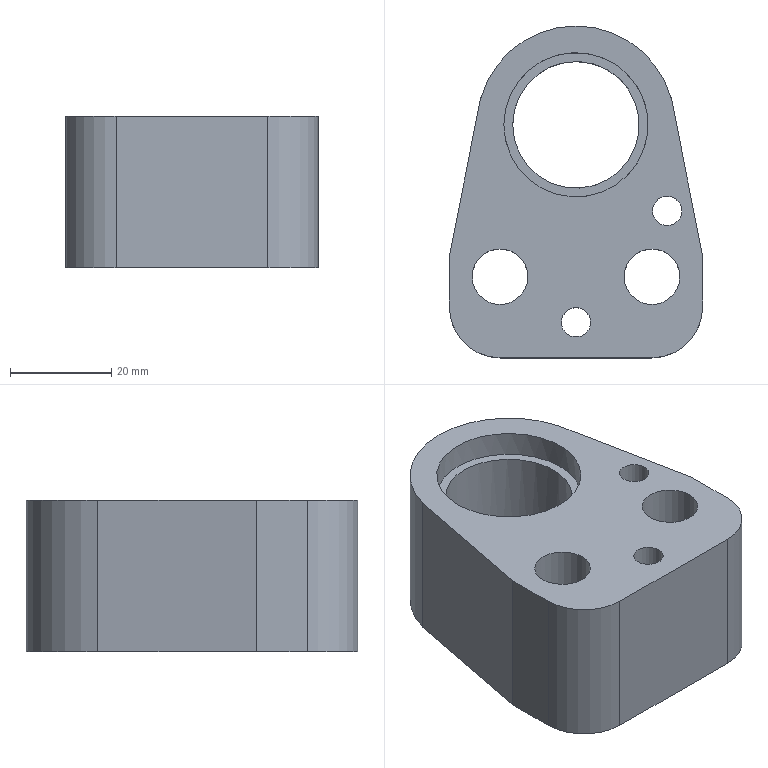Part | NX | features solid 2 | 1 solid | 27 faces | box 50 x 65.5 x 30 mm | volume 54795 mm3 | plane 14 | cylinder 13 | commonest cylinder face diameters 5.8 x2 8 x2 11 x2 17 x2 20 x2 25 x1
STEP:
#1=CARTESIAN_POINT('',(133.569,-304.452,65.));
#2=VERTEX_POINT('',#1);
#3=CARTESIAN_POINT('',(133.569,-304.452,95.));
#4=VERTEX_POINT('',#3);
#5=CARTESIAN_POINT('',(133.569,-304.452,65.));
#6=DIRECTION('',(0.,0.,1.));
#7=VECTOR('',#6,1000.);
#8=LINE('',#5,#7);
#9=EDGE_CURVE('',#2,#4,#8,.T.);
#10=ORIENTED_EDGE('',*,*,#9,.F.);
#11=CARTESIAN_POINT('',(133.497,-304.452,65.));
#12=VERTEX_POINT('',#11);
#13=CARTESIAN_POINT('',(114.754,-304.452,65.));
#14=DIRECTION('',(-1.,0.,0.));
#15=VECTOR('',#14,1000.);
#16=LINE('',#13,#15);
#17=EDGE_CURVE('',#2,#12,#16,.T.);
#18=ORIENTED_EDGE('',*,*,#17,.T.);
#19=CARTESIAN_POINT('',(133.497,-304.452,95.));
#20=VERTEX_POINT('',#19);
#21=CARTESIAN_POINT('',(133.497,-304.452,95.));
#22=DIRECTION('',(0.,0.,-1.));
#23=VECTOR('',#22,1000.);
#24=LINE('',#21,#23);
#25=EDGE_CURVE('',#20,#12,#24,.T.);
#26=ORIENTED_EDGE('',*,*,#25,.F.);
#27=CARTESIAN_POINT('',(114.754,-304.452,95.));
#28=DIRECTION('',(1.,0.,0.));
#29=VECTOR('',#28,1000.);
#30=LINE('',#27,#29);
#31=EDGE_CURVE('',#20,#4,#30,.T.);
#32=ORIENTED_EDGE('',*,*,#31,.T.);
#33=EDGE_LOOP('',(#10,#18,#26,#32));
#34=FACE_BOUND('',#33,.T.);
#35=CARTESIAN_POINT('',(114.754,-304.452,65.));
#36=DIRECTION('',(0.,1.,0.));
#37=DIRECTION('',(0.,0.,1.));
#38=AXIS2_PLACEMENT_3D('',#35,#36,#37);
#39=PLANE('',#38);
#40=ADVANCED_FACE('',(#34),#39,.T.);
#41=CARTESIAN_POINT('',(139.754,-335.832,95.));
#42=VERTEX_POINT('',#41);
#43=CARTESIAN_POINT('',(135.886,-316.209,95.));
#44=DIRECTION('',(-0.1934,0.9811,0.));
#45=VECTOR('',#44,1000.);
#46=LINE('',#43,#45);
#47=EDGE_CURVE('',#42,#4,#46,.T.);
#48=ORIENTED_EDGE('',*,*,#47,.T.);
#49=ORIENTED_EDGE('',*,*,#31,.F.);
#50=CARTESIAN_POINT('',(96.011,-304.452,95.));
#51=VERTEX_POINT('',#50);
#52=CARTESIAN_POINT('',(114.754,-309.832,95.));
#53=DIRECTION('',(0.,0.,-1.));
#54=DIRECTION('',(-1.,0.,0.));
#55=AXIS2_PLACEMENT_3D('',#52,#53,#54);
#56=CIRCLE('',#55,19.5);
#57=EDGE_CURVE('',#51,#20,#56,.T.);
#58=ORIENTED_EDGE('',*,*,#57,.F.);
#59=CARTESIAN_POINT('',(95.939,-304.452,95.));
#60=VERTEX_POINT('',#59);
#61=CARTESIAN_POINT('',(114.754,-304.452,95.));
#62=DIRECTION('',(1.,0.,0.));
#63=VECTOR('',#62,1000.);
#64=LINE('',#61,#63);
#65=EDGE_CURVE('',#60,#51,#64,.T.);
#66=ORIENTED_EDGE('',*,*,#65,.F.);
#67=CARTESIAN_POINT('',(89.754,-335.832,95.));
#68=VERTEX_POINT('',#67);
#69=CARTESIAN_POINT('',(93.622,-316.209,95.));
#70=DIRECTION('',(-0.1934,-0.9811,0.));
#71=VECTOR('',#70,1000.);
#72=LINE('',#69,#71);
#73=EDGE_CURVE('',#60,#68,#72,.T.);
#74=ORIENTED_EDGE('',*,*,#73,.T.);
#75=CARTESIAN_POINT('',(89.754,-345.832,95.));
#76=VERTEX_POINT('',#75);
#77=CARTESIAN_POINT('',(89.754,-320.142,95.));
#78=DIRECTION('',(0.,1.,0.));
#79=VECTOR('',#78,1000.);
#80=LINE('',#77,#79);
#81=EDGE_CURVE('',#76,#68,#80,.T.);
#82=ORIENTED_EDGE('',*,*,#81,.F.);
#83=CARTESIAN_POINT('',(99.754,-355.832,95.));
#84=VERTEX_POINT('',#83);
#85=CARTESIAN_POINT('',(99.754,-345.832,95.));
#86=DIRECTION('',(0.,0.,1.));
#87=DIRECTION('',(1.,0.,0.));
#88=AXIS2_PLACEMENT_3D('',#85,#86,#87);
#89=CIRCLE('',#88,10.);
#90=EDGE_CURVE('',#76,#84,#89,.T.);
#91=ORIENTED_EDGE('',*,*,#90,.T.);
#92=CARTESIAN_POINT('',(129.754,-355.832,95.));
#93=VERTEX_POINT('',#92);
#94=CARTESIAN_POINT('',(114.754,-355.832,95.));
#95=DIRECTION('',(-1.,0.,0.));
#96=VECTOR('',#95,1000.);
#97=LINE('',#94,#96);
#98=EDGE_CURVE('',#93,#84,#97,.T.);
#99=ORIENTED_EDGE('',*,*,#98,.F.);
#100=CARTESIAN_POINT('',(139.754,-345.832,95.));
#101=VERTEX_POINT('',#100);
#102=CARTESIAN_POINT('',(129.754,-345.832,95.));
#103=DIRECTION('',(0.,0.,1.));
#104=DIRECTION('',(1.,0.,0.));
#105=AXIS2_PLACEMENT_3D('',#102,#103,#104);
#106=CIRCLE('',#105,10.);
#107=EDGE_CURVE('',#93,#101,#106,.T.);
#108=ORIENTED_EDGE('',*,*,#107,.T.);
#109=CARTESIAN_POINT('',(139.754,-320.142,95.));
#110=DIRECTION('',(0.,-1.,0.));
#111=VECTOR('',#110,1000.);
#112=LINE('',#109,#111);
#113=EDGE_CURVE('',#42,#101,#112,.T.);
#114=ORIENTED_EDGE('',*,*,#113,.F.);
#115=EDGE_LOOP('',(#48,#49,#58,#66,#74,#82,#91,#99,#108,#114));
#116=FACE_BOUND('',#115,.T.);
#117=CARTESIAN_POINT('',(111.854,-348.832,95.));
#118=VERTEX_POINT('',#117);
#119=CARTESIAN_POINT('',(114.754,-348.832,95.));
#120=DIRECTION('',(0.,0.,-1.));
#121=DIRECTION('',(-1.,0.,0.));
#122=AXIS2_PLACEMENT_3D('',#119,#120,#121);
#123=CIRCLE('',#122,2.9);
#124=EDGE_CURVE('',#118,#118,#123,.T.);
#125=ORIENTED_EDGE('',*,*,#124,.T.);
#126=EDGE_LOOP('',(#125));
#127=FACE_BOUND('',#126,.T.);
#128=CARTESIAN_POINT('',(129.854,-326.832,95.));
#129=VERTEX_POINT('',#128);
#130=CARTESIAN_POINT('',(132.754,-326.832,95.));
#131=DIRECTION('',(0.,0.,-1.));
#132=DIRECTION('',(-1.,0.,0.));
#133=AXIS2_PLACEMENT_3D('',#130,#131,#132);
#134=CIRCLE('',#133,2.9);
#135=EDGE_CURVE('',#129,#129,#134,.T.);
#136=ORIENTED_EDGE('',*,*,#135,.T.);
#137=EDGE_LOOP('',(#136));
#138=FACE_BOUND('',#137,.T.);
#139=CARTESIAN_POINT('',(124.254,-339.832,95.));
#140=VERTEX_POINT('',#139);
#141=CARTESIAN_POINT('',(129.754,-339.832,95.));
#142=DIRECTION('',(0.,0.,-1.));
#143=DIRECTION('',(-1.,0.,0.));
#144=AXIS2_PLACEMENT_3D('',#141,#142,#143);
#145=CIRCLE('',#144,5.5);
#146=EDGE_CURVE('',#140,#140,#145,.T.);
#147=ORIENTED_EDGE('',*,*,#146,.T.);
#148=EDGE_LOOP('',(#147));
#149=FACE_BOUND('',#148,.T.);
#150=CARTESIAN_POINT('',(94.254,-339.832,95.));
#151=VERTEX_POINT('',#150);
#152=CARTESIAN_POINT('',(99.754,-339.832,95.));
#153=DIRECTION('',(0.,0.,-1.));
#154=DIRECTION('',(-1.,0.,0.));
#155=AXIS2_PLACEMENT_3D('',#152,#153,#154);
#156=CIRCLE('',#155,5.5);
#157=EDGE_CURVE('',#151,#151,#156,.T.);
#158=ORIENTED_EDGE('',*,*,#157,.T.);
#159=EDGE_LOOP('',(#158));
#160=FACE_BOUND('',#159,.T.);
#161=CARTESIAN_POINT('',(100.504,-309.832,95.));
#162=VERTEX_POINT('',#161);
#163=CARTESIAN_POINT('',(114.754,-309.832,95.));
#164=DIRECTION('',(0.,0.,-1.));
#165=DIRECTION('',(-1.,0.,0.));
#166=AXIS2_PLACEMENT_3D('',#163,#164,#165);
#167=CIRCLE('',#166,14.25);
#168=EDGE_CURVE('',#162,#162,#167,.T.);
#169=ORIENTED_EDGE('',*,*,#168,.T.);
#170=EDGE_LOOP('',(#169));
#171=FACE_BOUND('',#170,.T.);
#172=CARTESIAN_POINT('',(114.754,-320.142,95.));
#173=DIRECTION('',(0.,0.,1.));
#174=DIRECTION('',(1.,0.,0.));
#175=AXIS2_PLACEMENT_3D('',#172,#173,#174);
#176=PLANE('',#175);
#177=ADVANCED_FACE('',(#116,#127,#138,#149,#160,#171),#176,.T.);
#178=CARTESIAN_POINT('',(89.754,-335.832,65.));
#179=VERTEX_POINT('',#178);
#180=CARTESIAN_POINT('',(89.754,-335.832,65.));
#181=DIRECTION('',(0.,0.,1.));
#182=VECTOR('',#181,1000.);
#183=LINE('',#180,#182);
#184=EDGE_CURVE('',#179,#68,#183,.T.);
#185=ORIENTED_EDGE('',*,*,#184,.F.);
#186=CARTESIAN_POINT('',(89.754,-345.832,65.));
#187=VERTEX_POINT('',#186);
#188=CARTESIAN_POINT('',(89.754,-320.142,65.));
#189=DIRECTION('',(0.,-1.,0.));
#190=VECTOR('',#189,1000.);
#191=LINE('',#188,#190);
#192=EDGE_CURVE('',#179,#187,#191,.T.);
#193=ORIENTED_EDGE('',*,*,#192,.T.);
#194=CARTESIAN_POINT('',(89.754,-345.832,65.));
#195=DIRECTION('',(0.,0.,1.));
#196=VECTOR('',#195,1000.);
#197=LINE('',#194,#196);
#198=EDGE_CURVE('',#187,#76,#197,.T.);
#199=ORIENTED_EDGE('',*,*,#198,.T.);
#200=ORIENTED_EDGE('',*,*,#81,.T.);
#201=EDGE_LOOP('',(#185,#193,#199,#200));
#202=FACE_BOUND('',#201,.T.);
#203=CARTESIAN_POINT('',(89.754,-320.142,65.));
#204=DIRECTION('',(-1.,0.,0.));
#205=DIRECTION('',(0.,0.,1.));
#206=AXIS2_PLACEMENT_3D('',#203,#204,#205);
#207=PLANE('',#206);
#208=ADVANCED_FACE('',(#202),#207,.T.);
#209=CARTESIAN_POINT('',(95.939,-304.452,65.));
#210=VERTEX_POINT('',#209);
#211=CARTESIAN_POINT('',(95.939,-304.452,65.));
#212=DIRECTION('',(0.,0.,-1.));
#213=VECTOR('',#212,1000.);
#214=LINE('',#211,#213);
#215=EDGE_CURVE('',#60,#210,#214,.T.);
#216=ORIENTED_EDGE('',*,*,#215,.F.);
#217=ORIENTED_EDGE('',*,*,#65,.T.);
#218=CARTESIAN_POINT('',(96.011,-304.452,65.));
#219=VERTEX_POINT('',#218);
#220=CARTESIAN_POINT('',(96.011,-304.452,95.));
#221=DIRECTION('',(0.,0.,-1.));
#222=VECTOR('',#221,1000.);
#223=LINE('',#220,#222);
#224=EDGE_CURVE('',#219,#51,#223,.F.);
#225=ORIENTED_EDGE('',*,*,#224,.F.);
#226=CARTESIAN_POINT('',(114.754,-304.452,65.));
#227=DIRECTION('',(-1.,0.,0.));
#228=VECTOR('',#227,1000.);
#229=LINE('',#226,#228);
#230=EDGE_CURVE('',#219,#210,#229,.T.);
#231=ORIENTED_EDGE('',*,*,#230,.T.);
#232=EDGE_LOOP('',(#216,#217,#225,#231));
#233=FACE_BOUND('',#232,.T.);
#234=CARTESIAN_POINT('',(114.754,-304.452,65.));
#235=DIRECTION('',(0.,1.,0.));
#236=DIRECTION('',(0.,0.,1.));
#237=AXIS2_PLACEMENT_3D('',#234,#235,#236);
#238=PLANE('',#237);
#239=ADVANCED_FACE('',(#233),#238,.T.);
#240=CARTESIAN_POINT('',(139.754,-335.832,65.));
#241=VERTEX_POINT('',#240);
#242=CARTESIAN_POINT('',(135.886,-316.209,65.));
#243=DIRECTION('',(0.1934,-0.9811,0.));
#244=VECTOR('',#243,1000.);
#245=LINE('',#242,#244);
#246=EDGE_CURVE('',#2,#241,#245,.T.);
#247=ORIENTED_EDGE('',*,*,#246,.T.);
#248=CARTESIAN_POINT('',(139.754,-345.832,65.));
#249=VERTEX_POINT('',#248);
#250=CARTESIAN_POINT('',(139.754,-320.142,65.));
#251=DIRECTION('',(0.,1.,0.));
#252=VECTOR('',#251,1000.);
#253=LINE('',#250,#252);
#254=EDGE_CURVE('',#249,#241,#253,.T.);
#255=ORIENTED_EDGE('',*,*,#254,.F.);
#256=CARTESIAN_POINT('',(129.754,-355.832,65.));
#257=VERTEX_POINT('',#256);
#258=CARTESIAN_POINT('',(129.754,-345.832,65.));
#259=DIRECTION('',(0.,0.,-1.));
#260=DIRECTION('',(-1.,0.,0.));
#261=AXIS2_PLACEMENT_3D('',#258,#259,#260);
#262=CIRCLE('',#261,10.);
#263=EDGE_CURVE('',#249,#257,#262,.T.);
#264=ORIENTED_EDGE('',*,*,#263,.T.);
#265=CARTESIAN_POINT('',(99.754,-355.832,65.));
#266=VERTEX_POINT('',#265);
#267=CARTESIAN_POINT('',(114.754,-355.832,65.));
#268=DIRECTION('',(1.,0.,0.));
#269=VECTOR('',#268,1000.);
#270=LINE('',#267,#269);
#271=EDGE_CURVE('',#266,#257,#270,.T.);
#272=ORIENTED_EDGE('',*,*,#271,.F.);
#273=CARTESIAN_POINT('',(99.754,-345.832,65.));
#274=DIRECTION('',(0.,0.,-1.));
#275=DIRECTION('',(-1.,0.,0.));
#276=AXIS2_PLACEMENT_3D('',#273,#274,#275);
#277=CIRCLE('',#276,10.);
#278=EDGE_CURVE('',#266,#187,#277,.T.);
#279=ORIENTED_EDGE('',*,*,#278,.T.);
#280=ORIENTED_EDGE('',*,*,#192,.F.);
#281=CARTESIAN_POINT('',(93.622,-316.209,65.));
#282=DIRECTION('',(0.1934,0.9811,0.));
#283=VECTOR('',#282,1000.);
#284=LINE('',#281,#283);
#285=EDGE_CURVE('',#179,#210,#284,.T.);
#286=ORIENTED_EDGE('',*,*,#285,.T.);
#287=ORIENTED_EDGE('',*,*,#230,.F.);
#288=CARTESIAN_POINT('',(114.754,-309.832,65.));
#289=DIRECTION('',(0.,0.,1.));
#290=DIRECTION('',(1.,0.,0.));
#291=AXIS2_PLACEMENT_3D('',#288,#289,#290);
#292=CIRCLE('',#291,19.5);
#293=EDGE_CURVE('',#12,#219,#292,.T.);
#294=ORIENTED_EDGE('',*,*,#293,.F.);
#295=ORIENTED_EDGE('',*,*,#17,.F.);
#296=EDGE_LOOP('',(#247,#255,#264,#272,#279,#280,#286,#287,#294,#295));
#297=FACE_BOUND('',#296,.T.);
#298=CARTESIAN_POINT('',(118.754,-348.832,65.));
#299=VERTEX_POINT('',#298);
#300=CARTESIAN_POINT('',(114.754,-348.832,65.));
#301=DIRECTION('',(0.,0.,1.));
#302=DIRECTION('',(1.,0.,0.));
#303=AXIS2_PLACEMENT_3D('',#300,#301,#302);
#304=CIRCLE('',#303,4.);
#305=EDGE_CURVE('',#299,#299,#304,.T.);
#306=ORIENTED_EDGE('',*,*,#305,.T.);
#307=EDGE_LOOP('',(#306));
#308=FACE_BOUND('',#307,.T.);
#309=CARTESIAN_POINT('',(136.754,-326.832,65.));
#310=VERTEX_POINT('',#309);
#311=CARTESIAN_POINT('',(132.754,-326.832,65.));
#312=DIRECTION('',(0.,0.,1.));
#313=DIRECTION('',(1.,0.,0.));
#314=AXIS2_PLACEMENT_3D('',#311,#312,#313);
#315=CIRCLE('',#314,4.);
#316=EDGE_CURVE('',#310,#310,#315,.T.);
#317=ORIENTED_EDGE('',*,*,#316,.T.);
#318=EDGE_LOOP('',(#317));
#319=FACE_BOUND('',#318,.T.);
#320=CARTESIAN_POINT('',(138.254,-339.832,65.));
#321=VERTEX_POINT('',#320);
#322=CARTESIAN_POINT('',(129.754,-339.832,65.));
#323=DIRECTION('',(0.,0.,1.));
#324=DIRECTION('',(1.,0.,0.));
#325=AXIS2_PLACEMENT_3D('',#322,#323,#324);
#326=CIRCLE('',#325,8.5);
#327=EDGE_CURVE('',#321,#321,#326,.T.);
#328=ORIENTED_EDGE('',*,*,#327,.T.);
#329=EDGE_LOOP('',(#328));
#330=FACE_BOUND('',#329,.T.);
#331=CARTESIAN_POINT('',(108.254,-339.832,65.));
#332=VERTEX_POINT('',#331);
#333=CARTESIAN_POINT('',(99.754,-339.832,65.));
#334=DIRECTION('',(0.,0.,1.));
#335=DIRECTION('',(1.,0.,0.));
#336=AXIS2_PLACEMENT_3D('',#333,#334,#335);
#337=CIRCLE('',#336,8.5);
#338=EDGE_CURVE('',#332,#332,#337,.T.);
#339=ORIENTED_EDGE('',*,*,#338,.T.);
#340=EDGE_LOOP('',(#339));
#341=FACE_BOUND('',#340,.T.);
#342=CARTESIAN_POINT('',(127.254,-309.832,65.));
#343=VERTEX_POINT('',#342);
#344=CARTESIAN_POINT('',(114.754,-309.832,65.));
#345=DIRECTION('',(0.,0.,1.));
#346=DIRECTION('',(1.,0.,0.));
#347=AXIS2_PLACEMENT_3D('',#344,#345,#346);
#348=CIRCLE('',#347,12.5);
#349=EDGE_CURVE('',#343,#343,#348,.T.);
#350=ORIENTED_EDGE('',*,*,#349,.T.);
#351=EDGE_LOOP('',(#350));
#352=FACE_BOUND('',#351,.T.);
#353=CARTESIAN_POINT('',(114.754,-320.142,65.));
#354=DIRECTION('',(0.,0.,-1.));
#355=DIRECTION('',(-1.,0.,0.));
#356=AXIS2_PLACEMENT_3D('',#353,#354,#355);
#357=PLANE('',#356);
#358=ADVANCED_FACE('',(#297,#308,#319,#330,#341,#352),#357,.T.);
#359=CARTESIAN_POINT('',(139.754,-335.832,65.));
#360=DIRECTION('',(0.,0.,1.));
#361=VECTOR('',#360,1000.);
#362=LINE('',#359,#361);
#363=EDGE_CURVE('',#241,#42,#362,.T.);
#364=ORIENTED_EDGE('',*,*,#363,.T.);
#365=ORIENTED_EDGE('',*,*,#113,.T.);
#366=CARTESIAN_POINT('',(139.754,-345.832,65.));
#367=DIRECTION('',(0.,0.,1.));
#368=VECTOR('',#367,1000.);
#369=LINE('',#366,#368);
#370=EDGE_CURVE('',#101,#249,#369,.F.);
#371=ORIENTED_EDGE('',*,*,#370,.T.);
#372=ORIENTED_EDGE('',*,*,#254,.T.);
#373=EDGE_LOOP('',(#364,#365,#371,#372));
#374=FACE_BOUND('',#373,.T.);
#375=CARTESIAN_POINT('',(139.754,-320.142,65.));
#376=DIRECTION('',(1.,0.,0.));
#377=DIRECTION('',(0.,0.,-1.));
#378=AXIS2_PLACEMENT_3D('',#375,#376,#377);
#379=PLANE('',#378);
#380=ADVANCED_FACE('',(#374),#379,.T.);
#381=ORIENTED_EDGE('',*,*,#57,.T.);
#382=ORIENTED_EDGE('',*,*,#25,.T.);
#383=ORIENTED_EDGE('',*,*,#293,.T.);
#384=ORIENTED_EDGE('',*,*,#224,.T.);
#385=EDGE_LOOP('',(#381,#382,#383,#384));
#386=FACE_BOUND('',#385,.T.);
#387=CARTESIAN_POINT('',(114.754,-309.832,95.));
#388=DIRECTION('',(0.,0.,-1.));
#389=DIRECTION('',(-1.,0.,0.));
#390=AXIS2_PLACEMENT_3D('',#387,#388,#389);
#391=CYLINDRICAL_SURFACE('',#390,19.5);
#392=ADVANCED_FACE('',(#386),#391,.T.);
#393=ORIENTED_EDGE('',*,*,#271,.T.);
#394=CARTESIAN_POINT('',(129.754,-355.832,65.));
#395=DIRECTION('',(0.,0.,1.));
#396=VECTOR('',#395,1000.);
#397=LINE('',#394,#396);
#398=EDGE_CURVE('',#257,#93,#397,.T.);
#399=ORIENTED_EDGE('',*,*,#398,.T.);
#400=ORIENTED_EDGE('',*,*,#98,.T.);
#401=CARTESIAN_POINT('',(99.754,-355.832,65.));
#402=DIRECTION('',(0.,0.,1.));
#403=VECTOR('',#402,1000.);
#404=LINE('',#401,#403);
#405=EDGE_CURVE('',#84,#266,#404,.F.);
#406=ORIENTED_EDGE('',*,*,#405,.T.);
#407=EDGE_LOOP('',(#393,#399,#400,#406));
#408=FACE_BOUND('',#407,.T.);
#409=CARTESIAN_POINT('',(114.754,-355.832,65.));
#410=DIRECTION('',(0.,-1.,0.));
#411=DIRECTION('',(0.,0.,-1.));
#412=AXIS2_PLACEMENT_3D('',#409,#410,#411);
#413=PLANE('',#412);
#414=ADVANCED_FACE('',(#408),#413,.T.);
#415=CARTESIAN_POINT('',(102.254,-309.832,90.));
#416=VERTEX_POINT('',#415);
#417=CARTESIAN_POINT('',(114.754,-309.832,90.));
#418=DIRECTION('',(0.,0.,-1.));
#419=DIRECTION('',(-1.,0.,0.));
#420=AXIS2_PLACEMENT_3D('',#417,#418,#419);
#421=CIRCLE('',#420,12.5);
#422=EDGE_CURVE('',#416,#416,#421,.T.);
#423=ORIENTED_EDGE('',*,*,#422,.T.);
#424=EDGE_LOOP('',(#423));
#425=FACE_BOUND('',#424,.T.);
#426=CARTESIAN_POINT('',(129.004,-309.832,90.));
#427=VERTEX_POINT('',#426);
#428=CARTESIAN_POINT('',(114.754,-309.832,90.));
#429=DIRECTION('',(0.,0.,1.));
#430=DIRECTION('',(1.,0.,0.));
#431=AXIS2_PLACEMENT_3D('',#428,#429,#430);
#432=CIRCLE('',#431,14.25);
#433=EDGE_CURVE('',#427,#427,#432,.T.);
#434=ORIENTED_EDGE('',*,*,#433,.T.);
#435=EDGE_LOOP('',(#434));
#436=FACE_BOUND('',#435,.T.);
#437=CARTESIAN_POINT('',(114.754,-309.832,90.));
#438=DIRECTION('',(0.,0.,-1.));
#439=DIRECTION('',(-1.,0.,0.));
#440=AXIS2_PLACEMENT_3D('',#437,#438,#439);
#441=PLANE('',#440);
#442=ADVANCED_FACE('',(#425,#436),#441,.F.);
#443=ORIENTED_EDGE('',*,*,#433,.F.);
#444=EDGE_LOOP('',(#443));
#445=FACE_BOUND('',#444,.T.);
#446=ORIENTED_EDGE('',*,*,#168,.F.);
#447=EDGE_LOOP('',(#446));
#448=FACE_BOUND('',#447,.T.);
#449=CARTESIAN_POINT('',(114.754,-309.832,95.));
#450=DIRECTION('',(0.,0.,-1.));
#451=DIRECTION('',(-1.,0.,0.));
#452=AXIS2_PLACEMENT_3D('',#449,#450,#451);
#453=CYLINDRICAL_SURFACE('',#452,14.25);
#454=ADVANCED_FACE('',(#445,#448),#453,.F.);
#455=ORIENTED_EDGE('',*,*,#349,.F.);
#456=EDGE_LOOP('',(#455));
#457=FACE_BOUND('',#456,.T.);
#458=ORIENTED_EDGE('',*,*,#422,.F.);
#459=EDGE_LOOP('',(#458));
#460=FACE_BOUND('',#459,.T.);
#461=CARTESIAN_POINT('',(114.754,-309.832,90.));
#462=DIRECTION('',(0.,0.,-1.));
#463=DIRECTION('',(-1.,0.,0.));
#464=AXIS2_PLACEMENT_3D('',#461,#462,#463);
#465=CYLINDRICAL_SURFACE('',#464,12.5);
#466=ADVANCED_FACE('',(#457,#460),#465,.F.);
#467=CARTESIAN_POINT('',(105.254,-339.832,77.));
#468=VERTEX_POINT('',#467);
#469=CARTESIAN_POINT('',(99.754,-339.832,77.));
#470=DIRECTION('',(0.,0.,1.));
#471=DIRECTION('',(1.,0.,0.));
#472=AXIS2_PLACEMENT_3D('',#469,#470,#471);
#473=CIRCLE('',#472,5.5);
#474=EDGE_CURVE('',#468,#468,#473,.F.);
#475=ORIENTED_EDGE('',*,*,#474,.T.);
#476=EDGE_LOOP('',(#475));
#477=FACE_BOUND('',#476,.T.);
#478=ORIENTED_EDGE('',*,*,#157,.F.);
#479=EDGE_LOOP('',(#478));
#480=FACE_BOUND('',#479,.T.);
#481=CARTESIAN_POINT('',(99.754,-339.832,95.));
#482=DIRECTION('',(0.,0.,-1.));
#483=DIRECTION('',(-1.,0.,0.));
#484=AXIS2_PLACEMENT_3D('',#481,#482,#483);
#485=CYLINDRICAL_SURFACE('',#484,5.5);
#486=ADVANCED_FACE('',(#477,#480),#485,.F.);
#487=CARTESIAN_POINT('',(91.254,-339.832,77.));
#488=VERTEX_POINT('',#487);
#489=CARTESIAN_POINT('',(99.754,-339.832,77.));
#490=DIRECTION('',(0.,0.,-1.));
#491=DIRECTION('',(-1.,0.,0.));
#492=AXIS2_PLACEMENT_3D('',#489,#490,#491);
#493=CIRCLE('',#492,8.5);
#494=EDGE_CURVE('',#488,#488,#493,.T.);
#495=ORIENTED_EDGE('',*,*,#494,.T.);
#496=EDGE_LOOP('',(#495));
#497=FACE_BOUND('',#496,.T.);
#498=ORIENTED_EDGE('',*,*,#474,.F.);
#499=EDGE_LOOP('',(#498));
#500=FACE_BOUND('',#499,.T.);
#501=CARTESIAN_POINT('',(99.754,-339.832,77.));
#502=DIRECTION('',(0.,0.,1.));
#503=DIRECTION('',(1.,0.,0.));
#504=AXIS2_PLACEMENT_3D('',#501,#502,#503);
#505=PLANE('',#504);
#506=ADVANCED_FACE('',(#497,#500),#505,.F.);
#507=ORIENTED_EDGE('',*,*,#338,.F.);
#508=EDGE_LOOP('',(#507));
#509=FACE_BOUND('',#508,.T.);
#510=ORIENTED_EDGE('',*,*,#494,.F.);
#511=EDGE_LOOP('',(#510));
#512=FACE_BOUND('',#511,.T.);
#513=CARTESIAN_POINT('',(99.754,-339.832,77.));
#514=DIRECTION('',(0.,0.,-1.));
#515=DIRECTION('',(-1.,0.,0.));
#516=AXIS2_PLACEMENT_3D('',#513,#514,#515);
#517=CYLINDRICAL_SURFACE('',#516,8.5);
#518=ADVANCED_FACE('',(#509,#512),#517,.F.);
#519=CARTESIAN_POINT('',(135.254,-339.832,77.));
#520=VERTEX_POINT('',#519);
#521=CARTESIAN_POINT('',(129.754,-339.832,77.));
#522=DIRECTION('',(0.,0.,1.));
#523=DIRECTION('',(1.,0.,0.));
#524=AXIS2_PLACEMENT_3D('',#521,#522,#523);
#525=CIRCLE('',#524,5.5);
#526=EDGE_CURVE('',#520,#520,#525,.F.);
#527=ORIENTED_EDGE('',*,*,#526,.T.);
#528=EDGE_LOOP('',(#527));
#529=FACE_BOUND('',#528,.T.);
#530=ORIENTED_EDGE('',*,*,#146,.F.);
#531=EDGE_LOOP('',(#530));
#532=FACE_BOUND('',#531,.T.);
#533=CARTESIAN_POINT('',(129.754,-339.832,95.));
#534=DIRECTION('',(0.,0.,-1.));
#535=DIRECTION('',(-1.,0.,0.));
#536=AXIS2_PLACEMENT_3D('',#533,#534,#535);
#537=CYLINDRICAL_SURFACE('',#536,5.5);
#538=ADVANCED_FACE('',(#529,#532),#537,.F.);
#539=CARTESIAN_POINT('',(121.254,-339.832,77.));
#540=VERTEX_POINT('',#539);
#541=CARTESIAN_POINT('',(129.754,-339.832,77.));
#542=DIRECTION('',(0.,0.,-1.));
#543=DIRECTION('',(-1.,0.,0.));
#544=AXIS2_PLACEMENT_3D('',#541,#542,#543);
#545=CIRCLE('',#544,8.5);
#546=EDGE_CURVE('',#540,#540,#545,.T.);
#547=ORIENTED_EDGE('',*,*,#546,.T.);
#548=EDGE_LOOP('',(#547));
#549=FACE_BOUND('',#548,.T.);
#550=ORIENTED_EDGE('',*,*,#526,.F.);
#551=EDGE_LOOP('',(#550));
#552=FACE_BOUND('',#551,.T.);
#553=CARTESIAN_POINT('',(129.754,-339.832,77.));
#554=DIRECTION('',(0.,0.,1.));
#555=DIRECTION('',(1.,0.,0.));
#556=AXIS2_PLACEMENT_3D('',#553,#554,#555);
#557=PLANE('',#556);
#558=ADVANCED_FACE('',(#549,#552),#557,.F.);
#559=ORIENTED_EDGE('',*,*,#327,.F.);
#560=EDGE_LOOP('',(#559));
#561=FACE_BOUND('',#560,.T.);
#562=ORIENTED_EDGE('',*,*,#546,.F.);
#563=EDGE_LOOP('',(#562));
#564=FACE_BOUND('',#563,.T.);
#565=CARTESIAN_POINT('',(129.754,-339.832,77.));
#566=DIRECTION('',(0.,0.,-1.));
#567=DIRECTION('',(-1.,0.,0.));
#568=AXIS2_PLACEMENT_3D('',#565,#566,#567);
#569=CYLINDRICAL_SURFACE('',#568,8.5);
#570=ADVANCED_FACE('',(#561,#564),#569,.F.);
#571=CARTESIAN_POINT('',(135.654,-326.832,85.));
#572=VERTEX_POINT('',#571);
#573=CARTESIAN_POINT('',(132.754,-326.832,85.));
#574=DIRECTION('',(0.,0.,1.));
#575=DIRECTION('',(1.,0.,0.));
#576=AXIS2_PLACEMENT_3D('',#573,#574,#575);
#577=CIRCLE('',#576,2.9);
#578=EDGE_CURVE('',#572,#572,#577,.F.);
#579=ORIENTED_EDGE('',*,*,#578,.T.);
#580=EDGE_LOOP('',(#579));
#581=FACE_BOUND('',#580,.T.);
#582=ORIENTED_EDGE('',*,*,#135,.F.);
#583=EDGE_LOOP('',(#582));
#584=FACE_BOUND('',#583,.T.);
#585=CARTESIAN_POINT('',(132.754,-326.832,95.));
#586=DIRECTION('',(0.,0.,-1.));
#587=DIRECTION('',(-1.,0.,0.));
#588=AXIS2_PLACEMENT_3D('',#585,#586,#587);
#589=CYLINDRICAL_SURFACE('',#588,2.9);
#590=ADVANCED_FACE('',(#581,#584),#589,.F.);
#591=CARTESIAN_POINT('',(128.754,-326.832,85.));
#592=VERTEX_POINT('',#591);
#593=CARTESIAN_POINT('',(132.754,-326.832,85.));
#594=DIRECTION('',(0.,0.,-1.));
#595=DIRECTION('',(-1.,0.,0.));
#596=AXIS2_PLACEMENT_3D('',#593,#594,#595);
#597=CIRCLE('',#596,4.);
#598=EDGE_CURVE('',#592,#592,#597,.T.);
#599=ORIENTED_EDGE('',*,*,#598,.T.);
#600=EDGE_LOOP('',(#599));
#601=FACE_BOUND('',#600,.T.);
#602=ORIENTED_EDGE('',*,*,#578,.F.);
#603=EDGE_LOOP('',(#602));
#604=FACE_BOUND('',#603,.T.);
#605=CARTESIAN_POINT('',(132.754,-326.832,85.));
#606=DIRECTION('',(0.,0.,1.));
#607=DIRECTION('',(1.,0.,0.));
#608=AXIS2_PLACEMENT_3D('',#605,#606,#607);
#609=PLANE('',#608);
#610=ADVANCED_FACE('',(#601,#604),#609,.F.);
#611=ORIENTED_EDGE('',*,*,#316,.F.);
#612=EDGE_LOOP('',(#611));
#613=FACE_BOUND('',#612,.T.);
#614=ORIENTED_EDGE('',*,*,#598,.F.);
#615=EDGE_LOOP('',(#614));
#616=FACE_BOUND('',#615,.T.);
#617=CARTESIAN_POINT('',(132.754,-326.832,85.));
#618=DIRECTION('',(0.,0.,-1.));
#619=DIRECTION('',(-1.,0.,0.));
#620=AXIS2_PLACEMENT_3D('',#617,#618,#619);
#621=CYLINDRICAL_SURFACE('',#620,4.);
#622=ADVANCED_FACE('',(#613,#616),#621,.F.);
#623=CARTESIAN_POINT('',(117.654,-348.832,85.));
#624=VERTEX_POINT('',#623);
#625=CARTESIAN_POINT('',(114.754,-348.832,85.));
#626=DIRECTION('',(0.,0.,1.));
#627=DIRECTION('',(1.,0.,0.));
#628=AXIS2_PLACEMENT_3D('',#625,#626,#627);
#629=CIRCLE('',#628,2.9);
#630=EDGE_CURVE('',#624,#624,#629,.F.);
#631=ORIENTED_EDGE('',*,*,#630,.T.);
#632=EDGE_LOOP('',(#631));
#633=FACE_BOUND('',#632,.T.);
#634=ORIENTED_EDGE('',*,*,#124,.F.);
#635=EDGE_LOOP('',(#634));
#636=FACE_BOUND('',#635,.T.);
#637=CARTESIAN_POINT('',(114.754,-348.832,95.));
#638=DIRECTION('',(0.,0.,-1.));
#639=DIRECTION('',(-1.,0.,0.));
#640=AXIS2_PLACEMENT_3D('',#637,#638,#639);
#641=CYLINDRICAL_SURFACE('',#640,2.9);
#642=ADVANCED_FACE('',(#633,#636),#641,.F.);
#643=CARTESIAN_POINT('',(110.754,-348.832,85.));
#644=VERTEX_POINT('',#643);
#645=CARTESIAN_POINT('',(114.754,-348.832,85.));
#646=DIRECTION('',(0.,0.,-1.));
#647=DIRECTION('',(-1.,0.,0.));
#648=AXIS2_PLACEMENT_3D('',#645,#646,#647);
#649=CIRCLE('',#648,4.);
#650=EDGE_CURVE('',#644,#644,#649,.T.);
#651=ORIENTED_EDGE('',*,*,#650,.T.);
#652=EDGE_LOOP('',(#651));
#653=FACE_BOUND('',#652,.T.);
#654=ORIENTED_EDGE('',*,*,#630,.F.);
#655=EDGE_LOOP('',(#654));
#656=FACE_BOUND('',#655,.T.);
#657=CARTESIAN_POINT('',(114.754,-348.832,85.));
#658=DIRECTION('',(0.,0.,1.));
#659=DIRECTION('',(1.,0.,0.));
#660=AXIS2_PLACEMENT_3D('',#657,#658,#659);
#661=PLANE('',#660);
#662=ADVANCED_FACE('',(#653,#656),#661,.F.);
#663=ORIENTED_EDGE('',*,*,#305,.F.);
#664=EDGE_LOOP('',(#663));
#665=FACE_BOUND('',#664,.T.);
#666=ORIENTED_EDGE('',*,*,#650,.F.);
#667=EDGE_LOOP('',(#666));
#668=FACE_BOUND('',#667,.T.);
#669=CARTESIAN_POINT('',(114.754,-348.832,85.));
#670=DIRECTION('',(0.,0.,-1.));
#671=DIRECTION('',(-1.,0.,0.));
#672=AXIS2_PLACEMENT_3D('',#669,#670,#671);
#673=CYLINDRICAL_SURFACE('',#672,4.);
#674=ADVANCED_FACE('',(#665,#668),#673,.F.);
#675=ORIENTED_EDGE('',*,*,#263,.F.);
#676=ORIENTED_EDGE('',*,*,#370,.F.);
#677=ORIENTED_EDGE('',*,*,#107,.F.);
#678=ORIENTED_EDGE('',*,*,#398,.F.);
#679=EDGE_LOOP('',(#675,#676,#677,#678));
#680=FACE_BOUND('',#679,.T.);
#681=CARTESIAN_POINT('',(129.754,-345.832,65.));
#682=DIRECTION('',(0.,0.,1.));
#683=DIRECTION('',(1.,0.,0.));
#684=AXIS2_PLACEMENT_3D('',#681,#682,#683);
#685=CYLINDRICAL_SURFACE('',#684,10.);
#686=ADVANCED_FACE('',(#680),#685,.T.);
#687=ORIENTED_EDGE('',*,*,#278,.F.);
#688=ORIENTED_EDGE('',*,*,#405,.F.);
#689=ORIENTED_EDGE('',*,*,#90,.F.);
#690=ORIENTED_EDGE('',*,*,#198,.F.);
#691=EDGE_LOOP('',(#687,#688,#689,#690));
#692=FACE_BOUND('',#691,.T.);
#693=CARTESIAN_POINT('',(99.754,-345.832,65.));
#694=DIRECTION('',(0.,0.,1.));
#695=DIRECTION('',(1.,0.,0.));
#696=AXIS2_PLACEMENT_3D('',#693,#694,#695);
#697=CYLINDRICAL_SURFACE('',#696,10.);
#698=ADVANCED_FACE('',(#692),#697,.T.);
#699=ORIENTED_EDGE('',*,*,#215,.T.);
#700=ORIENTED_EDGE('',*,*,#285,.F.);
#701=ORIENTED_EDGE('',*,*,#184,.T.);
#702=ORIENTED_EDGE('',*,*,#73,.F.);
#703=EDGE_LOOP('',(#699,#700,#701,#702));
#704=FACE_BOUND('',#703,.T.);
#705=CARTESIAN_POINT('',(93.622,-316.209,65.));
#706=DIRECTION('',(0.9811,-0.1934,0.));
#707=DIRECTION('',(0.,0.,-1.));
#708=AXIS2_PLACEMENT_3D('',#705,#706,#707);
#709=PLANE('',#708);
#710=ADVANCED_FACE('',(#704),#709,.F.);
#711=ORIENTED_EDGE('',*,*,#9,.T.);
#712=ORIENTED_EDGE('',*,*,#47,.F.);
#713=ORIENTED_EDGE('',*,*,#363,.F.);
#714=ORIENTED_EDGE('',*,*,#246,.F.);
#715=EDGE_LOOP('',(#711,#712,#713,#714));
#716=FACE_BOUND('',#715,.T.);
#717=CARTESIAN_POINT('',(135.886,-316.209,65.));
#718=DIRECTION('',(-0.9811,-0.1934,0.));
#719=DIRECTION('',(0.,0.,1.));
#720=AXIS2_PLACEMENT_3D('',#717,#718,#719);
#721=PLANE('',#720);
#722=ADVANCED_FACE('',(#716),#721,.F.);
#723=CLOSED_SHELL('',(#40,#177,#208,#239,#358,#380,#392,#414,#442,#454,#466,#486,#506,#518,#538,#558,#570,#590,#610,#622,#642,#662,#674,#686,#698,#710,#722));
#724=MANIFOLD_SOLID_BREP('',#723);
#725=(LENGTH_UNIT()NAMED_UNIT(*)SI_UNIT(.MILLI.,.METRE.));
#726=UNCERTAINTY_MEASURE_WITH_UNIT(LENGTH_MEASURE(0.00001),#725,'','');
#727=(NAMED_UNIT(*)PLANE_ANGLE_UNIT()SI_UNIT($,.RADIAN.));
#728=(NAMED_UNIT(*)SI_UNIT($,.STERADIAN.)SOLID_ANGLE_UNIT());
#729=(GEOMETRIC_REPRESENTATION_CONTEXT(3)GLOBAL_UNCERTAINTY_ASSIGNED_CONTEXT((#726))GLOBAL_UNIT_ASSIGNED_CONTEXT((#725,#727,#728))REPRESENTATION_CONTEXT('',''));
#730=ADVANCED_BREP_SHAPE_REPRESENTATION('',(#724),#729);